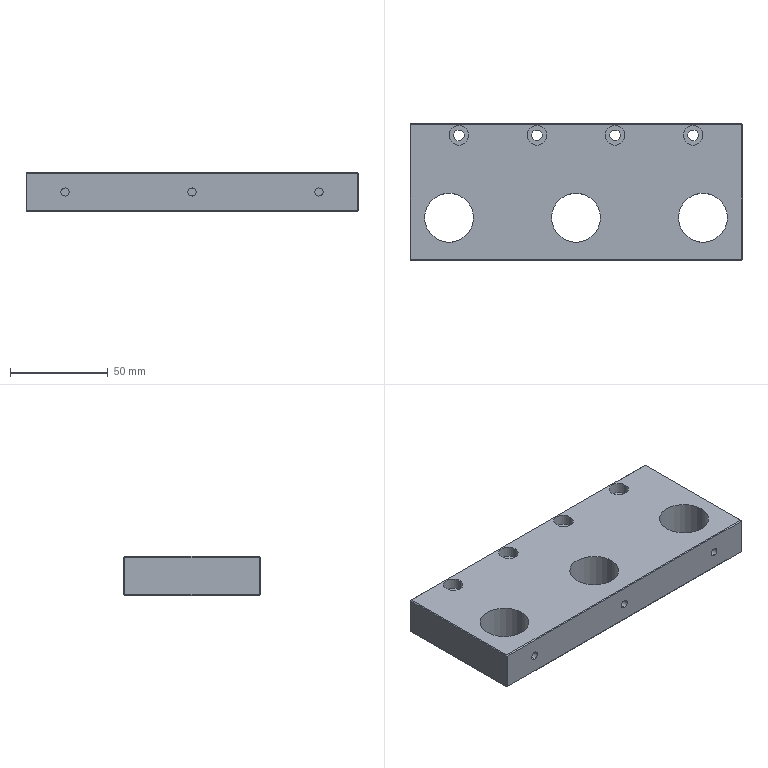Part | STEP file | 1 solid | 58 faces | box 170 x 70 x 20 mm | volume 204646 mm3 | plane 30 | cylinder 28 | commonest cylinder face diameters 5.5 x8 10 x8 4.2 x6 25.1 x6